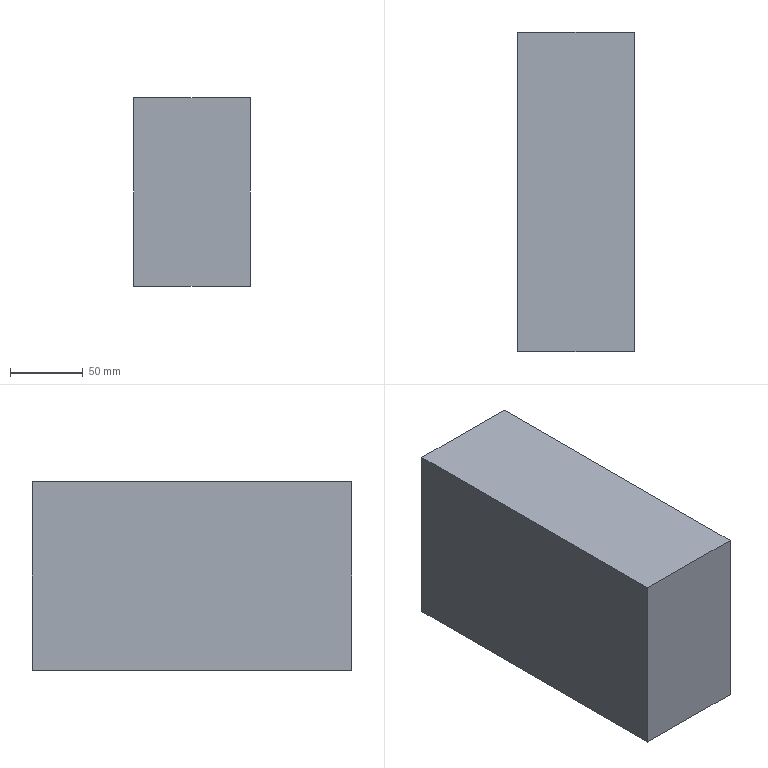Part | NX | features solid 2 | 1 solid | 6 faces | box 80 x 220 x 130 mm | volume 2288000 mm3 | plane 6
STEP:
#1=CARTESIAN_POINT('',(-1145.,-435.,-295.));
#2=VERTEX_POINT('',#1);
#3=CARTESIAN_POINT('',(-1145.,-215.,-295.));
#4=VERTEX_POINT('',#3);
#5=CARTESIAN_POINT('',(-1145.,-385.,-295.));
#6=DIRECTION('',(0.,1.,0.));
#7=VECTOR('',#6,1000.);
#8=LINE('',#5,#7);
#9=EDGE_CURVE('',#2,#4,#8,.T.);
#10=ORIENTED_EDGE('',*,*,#9,.F.);
#11=CARTESIAN_POINT('',(-1065.,-435.,-295.));
#12=VERTEX_POINT('',#11);
#13=CARTESIAN_POINT('',(-1075.,-435.,-295.));
#14=DIRECTION('',(-1.,0.,0.));
#15=VECTOR('',#14,1000.);
#16=LINE('',#13,#15);
#17=EDGE_CURVE('',#12,#2,#16,.T.);
#18=ORIENTED_EDGE('',*,*,#17,.F.);
#19=CARTESIAN_POINT('',(-1065.,-215.,-295.));
#20=VERTEX_POINT('',#19);
#21=CARTESIAN_POINT('',(-1065.,-385.,-295.));
#22=DIRECTION('',(0.,1.,0.));
#23=VECTOR('',#22,1000.);
#24=LINE('',#21,#23);
#25=EDGE_CURVE('',#12,#20,#24,.T.);
#26=ORIENTED_EDGE('',*,*,#25,.T.);
#27=CARTESIAN_POINT('',(-1075.,-215.,-295.));
#28=DIRECTION('',(-1.,0.,0.));
#29=VECTOR('',#28,1000.);
#30=LINE('',#27,#29);
#31=EDGE_CURVE('',#20,#4,#30,.T.);
#32=ORIENTED_EDGE('',*,*,#31,.T.);
#33=EDGE_LOOP('',(#10,#18,#26,#32));
#34=FACE_BOUND('',#33,.T.);
#35=CARTESIAN_POINT('',(-1075.,-385.,-295.));
#36=DIRECTION('',(0.,0.,1.));
#37=DIRECTION('',(1.,0.,0.));
#38=AXIS2_PLACEMENT_3D('',#35,#36,#37);
#39=PLANE('',#38);
#40=ADVANCED_FACE('',(#34),#39,.T.);
#41=CARTESIAN_POINT('',(-1145.,-215.,-425.));
#42=VERTEX_POINT('',#41);
#43=CARTESIAN_POINT('',(-1145.,-215.,-300.));
#44=DIRECTION('',(0.,0.,-1.));
#45=VECTOR('',#44,1000.);
#46=LINE('',#43,#45);
#47=EDGE_CURVE('',#4,#42,#46,.T.);
#48=ORIENTED_EDGE('',*,*,#47,.F.);
#49=ORIENTED_EDGE('',*,*,#31,.F.);
#50=CARTESIAN_POINT('',(-1065.,-215.,-425.));
#51=VERTEX_POINT('',#50);
#52=CARTESIAN_POINT('',(-1065.,-215.,-300.));
#53=DIRECTION('',(0.,0.,-1.));
#54=VECTOR('',#53,1000.);
#55=LINE('',#52,#54);
#56=EDGE_CURVE('',#20,#51,#55,.T.);
#57=ORIENTED_EDGE('',*,*,#56,.T.);
#58=CARTESIAN_POINT('',(-1075.,-215.,-425.));
#59=DIRECTION('',(-1.,0.,0.));
#60=VECTOR('',#59,1000.);
#61=LINE('',#58,#60);
#62=EDGE_CURVE('',#51,#42,#61,.T.);
#63=ORIENTED_EDGE('',*,*,#62,.T.);
#64=EDGE_LOOP('',(#48,#49,#57,#63));
#65=FACE_BOUND('',#64,.T.);
#66=CARTESIAN_POINT('',(-1075.,-215.,-300.));
#67=DIRECTION('',(0.,1.,0.));
#68=DIRECTION('',(0.,0.,1.));
#69=AXIS2_PLACEMENT_3D('',#66,#67,#68);
#70=PLANE('',#69);
#71=ADVANCED_FACE('',(#65),#70,.T.);
#72=CARTESIAN_POINT('',(-1145.,-435.,-425.));
#73=VERTEX_POINT('',#72);
#74=CARTESIAN_POINT('',(-1145.,-385.,-425.));
#75=DIRECTION('',(0.,1.,0.));
#76=VECTOR('',#75,1000.);
#77=LINE('',#74,#76);
#78=EDGE_CURVE('',#73,#42,#77,.T.);
#79=ORIENTED_EDGE('',*,*,#78,.T.);
#80=ORIENTED_EDGE('',*,*,#62,.F.);
#81=CARTESIAN_POINT('',(-1065.,-435.,-425.));
#82=VERTEX_POINT('',#81);
#83=CARTESIAN_POINT('',(-1065.,-385.,-425.));
#84=DIRECTION('',(0.,1.,0.));
#85=VECTOR('',#84,1000.);
#86=LINE('',#83,#85);
#87=EDGE_CURVE('',#82,#51,#86,.T.);
#88=ORIENTED_EDGE('',*,*,#87,.F.);
#89=CARTESIAN_POINT('',(-1075.,-435.,-425.));
#90=DIRECTION('',(-1.,0.,0.));
#91=VECTOR('',#90,1000.);
#92=LINE('',#89,#91);
#93=EDGE_CURVE('',#82,#73,#92,.T.);
#94=ORIENTED_EDGE('',*,*,#93,.T.);
#95=EDGE_LOOP('',(#79,#80,#88,#94));
#96=FACE_BOUND('',#95,.T.);
#97=CARTESIAN_POINT('',(-1075.,-385.,-425.));
#98=DIRECTION('',(0.,0.,1.));
#99=DIRECTION('',(1.,0.,0.));
#100=AXIS2_PLACEMENT_3D('',#97,#98,#99);
#101=PLANE('',#100);
#102=ADVANCED_FACE('',(#96),#101,.F.);
#103=CARTESIAN_POINT('',(-1145.,-435.,-300.));
#104=DIRECTION('',(0.,0.,-1.));
#105=VECTOR('',#104,1000.);
#106=LINE('',#103,#105);
#107=EDGE_CURVE('',#2,#73,#106,.T.);
#108=ORIENTED_EDGE('',*,*,#107,.T.);
#109=ORIENTED_EDGE('',*,*,#93,.F.);
#110=CARTESIAN_POINT('',(-1065.,-435.,-300.));
#111=DIRECTION('',(0.,0.,-1.));
#112=VECTOR('',#111,1000.);
#113=LINE('',#110,#112);
#114=EDGE_CURVE('',#12,#82,#113,.T.);
#115=ORIENTED_EDGE('',*,*,#114,.F.);
#116=ORIENTED_EDGE('',*,*,#17,.T.);
#117=EDGE_LOOP('',(#108,#109,#115,#116));
#118=FACE_BOUND('',#117,.T.);
#119=CARTESIAN_POINT('',(-1075.,-435.,-300.));
#120=DIRECTION('',(0.,1.,0.));
#121=DIRECTION('',(0.,0.,1.));
#122=AXIS2_PLACEMENT_3D('',#119,#120,#121);
#123=PLANE('',#122);
#124=ADVANCED_FACE('',(#118),#123,.F.);
#125=ORIENTED_EDGE('',*,*,#25,.F.);
#126=ORIENTED_EDGE('',*,*,#114,.T.);
#127=ORIENTED_EDGE('',*,*,#87,.T.);
#128=ORIENTED_EDGE('',*,*,#56,.F.);
#129=EDGE_LOOP('',(#125,#126,#127,#128));
#130=FACE_BOUND('',#129,.T.);
#131=CARTESIAN_POINT('',(-1065.,-385.,-300.));
#132=DIRECTION('',(-1.,0.,0.));
#133=DIRECTION('',(0.,0.,1.));
#134=AXIS2_PLACEMENT_3D('',#131,#132,#133);
#135=PLANE('',#134);
#136=ADVANCED_FACE('',(#130),#135,.F.);
#137=ORIENTED_EDGE('',*,*,#9,.T.);
#138=ORIENTED_EDGE('',*,*,#47,.T.);
#139=ORIENTED_EDGE('',*,*,#78,.F.);
#140=ORIENTED_EDGE('',*,*,#107,.F.);
#141=EDGE_LOOP('',(#137,#138,#139,#140));
#142=FACE_BOUND('',#141,.T.);
#143=CARTESIAN_POINT('',(-1145.,-385.,-300.));
#144=DIRECTION('',(-1.,0.,0.));
#145=DIRECTION('',(0.,0.,1.));
#146=AXIS2_PLACEMENT_3D('',#143,#144,#145);
#147=PLANE('',#146);
#148=ADVANCED_FACE('',(#142),#147,.T.);
#149=CLOSED_SHELL('',(#40,#71,#102,#124,#136,#148));
#150=MANIFOLD_SOLID_BREP('',#149);
#151=(LENGTH_UNIT()NAMED_UNIT(*)SI_UNIT(.MILLI.,.METRE.));
#152=UNCERTAINTY_MEASURE_WITH_UNIT(LENGTH_MEASURE(0.00001),#151,'','');
#153=(NAMED_UNIT(*)PLANE_ANGLE_UNIT()SI_UNIT($,.RADIAN.));
#154=(NAMED_UNIT(*)SI_UNIT($,.STERADIAN.)SOLID_ANGLE_UNIT());
#155=(GEOMETRIC_REPRESENTATION_CONTEXT(3)GLOBAL_UNCERTAINTY_ASSIGNED_CONTEXT((#152))GLOBAL_UNIT_ASSIGNED_CONTEXT((#151,#153,#154))REPRESENTATION_CONTEXT('',''));
#156=ADVANCED_BREP_SHAPE_REPRESENTATION('',(#150),#155);